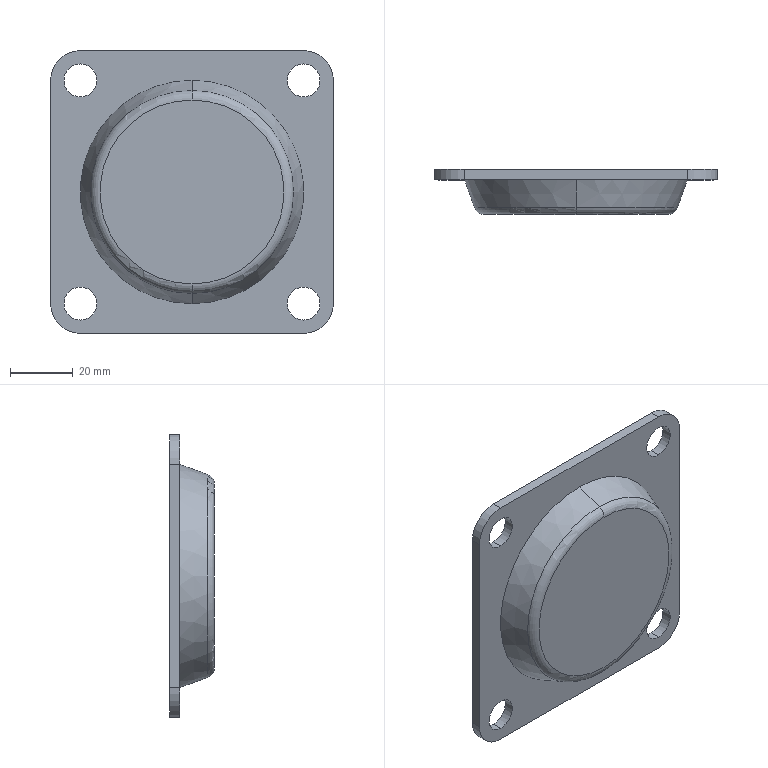Part | SolidWorks | features RefAxis 6, 3DProfileFeature 2, ICE 2, Extrusion 1, Revolution 1 | 1 solid | 29 faces | box 90 x 14.2 x 90 mm | volume 60346 mm3 | cylinder 16 | plane 9 | cone 2 | torus 2 | commonest cylinder face diameters 10.5 x8 19 x4 27 x2 54 x2
STEP:
#1=CARTESIAN_POINT('',(0.,-12.094,32.263));
#2=VERTEX_POINT('',#1);
#3=CARTESIAN_POINT('',(0.,-12.094,-32.263));
#4=VERTEX_POINT('',#3);
#5=CARTESIAN_POINT('',(0.,-12.094,0.));
#6=DIRECTION('',(0.,1.,0.));
#7=DIRECTION('',(0.,0.,1.));
#8=AXIS2_PLACEMENT_3D('',#5,#6,#7);
#9=CIRCLE('',#8,32.263);
#10=EDGE_CURVE('',#2,#4,#9,.T.);
#11=ORIENTED_EDGE('',*,*,#10,.T.);
#12=CARTESIAN_POINT('',(0.,-3.2,-35.5));
#13=VERTEX_POINT('',#12);
#14=CARTESIAN_POINT('',(0.,-3.2,-35.5));
#15=DIRECTION('',(0.,0.9397,-0.342));
#16=VECTOR('',#15,1000.);
#17=LINE('',#14,#16);
#18=EDGE_CURVE('',#4,#13,#17,.T.);
#19=ORIENTED_EDGE('',*,*,#18,.T.);
#20=CARTESIAN_POINT('',(0.,-3.2,35.5));
#21=VERTEX_POINT('',#20);
#22=CARTESIAN_POINT('',(0.,-3.2,0.));
#23=DIRECTION('',(0.,1.,0.));
#24=DIRECTION('',(0.,0.,1.));
#25=AXIS2_PLACEMENT_3D('',#22,#23,#24);
#26=CIRCLE('',#25,35.5);
#27=EDGE_CURVE('',#21,#13,#26,.T.);
#28=ORIENTED_EDGE('',*,*,#27,.F.);
#29=CARTESIAN_POINT('',(0.,-3.2,35.5));
#30=DIRECTION('',(0.,0.9397,0.342));
#31=VECTOR('',#30,1000.);
#32=LINE('',#29,#31);
#33=EDGE_CURVE('',#2,#21,#32,.T.);
#34=ORIENTED_EDGE('',*,*,#33,.F.);
#35=EDGE_LOOP('',(#11,#19,#28,#34));
#36=FACE_OUTER_BOUND('',#35,.T.);
#37=CARTESIAN_POINT('',(0.,-3.2,0.));
#38=DIRECTION('',(0.,1.,0.));
#39=DIRECTION('',(0.,0.,1.));
#40=AXIS2_PLACEMENT_3D('',#37,#38,#39);
#41=CONICAL_SURFACE('',#40,35.5,0.3491);
#42=ADVANCED_FACE('',(#36),#41,.T.);
#43=CARTESIAN_POINT('',(0.,-14.2,29.256));
#44=VERTEX_POINT('',#43);
#45=CARTESIAN_POINT('',(0.,-14.2,-29.256));
#46=VERTEX_POINT('',#45);
#47=CARTESIAN_POINT('',(0.,-14.2,0.));
#48=DIRECTION('',(0.,1.,0.));
#49=DIRECTION('',(0.,0.,1.));
#50=AXIS2_PLACEMENT_3D('',#47,#48,#49);
#51=CIRCLE('',#50,29.256);
#52=EDGE_CURVE('',#44,#46,#51,.T.);
#53=ORIENTED_EDGE('',*,*,#52,.T.);
#54=CARTESIAN_POINT('',(0.,-11.,-29.256));
#55=DIRECTION('',(1.,0.,0.));
#56=DIRECTION('',(0.,0.,-1.));
#57=AXIS2_PLACEMENT_3D('',#54,#55,#56);
#58=CIRCLE('',#57,3.2);
#59=EDGE_CURVE('',#46,#4,#58,.T.);
#60=ORIENTED_EDGE('',*,*,#59,.T.);
#61=ORIENTED_EDGE('',*,*,#10,.F.);
#62=CARTESIAN_POINT('',(0.,-11.,29.256));
#63=DIRECTION('',(-1.,0.,0.));
#64=DIRECTION('',(0.,0.,1.));
#65=AXIS2_PLACEMENT_3D('',#62,#63,#64);
#66=CIRCLE('',#65,3.2);
#67=EDGE_CURVE('',#44,#2,#66,.T.);
#68=ORIENTED_EDGE('',*,*,#67,.F.);
#69=EDGE_LOOP('',(#53,#60,#61,#68));
#70=FACE_OUTER_BOUND('',#69,.T.);
#71=CARTESIAN_POINT('',(0.,-11.,0.));
#72=DIRECTION('',(0.,1.,0.));
#73=DIRECTION('',(0.,0.,1.));
#74=AXIS2_PLACEMENT_3D('',#71,#72,#73);
#75=TOROIDAL_SURFACE('',#74,29.256,3.2);
#76=ADVANCED_FACE('',(#70),#75,.T.);
#77=CARTESIAN_POINT('',(0.,-0.5,13.5));
#78=VERTEX_POINT('',#77);
#79=CARTESIAN_POINT('',(0.,-0.5,-13.5));
#80=VERTEX_POINT('',#79);
#81=CARTESIAN_POINT('',(0.,-0.5,0.));
#82=DIRECTION('',(0.,1.,0.));
#83=DIRECTION('',(0.,0.,1.));
#84=AXIS2_PLACEMENT_3D('',#81,#82,#83);
#85=CIRCLE('',#84,13.5);
#86=EDGE_CURVE('',#78,#80,#85,.T.);
#87=ORIENTED_EDGE('',*,*,#86,.F.);
#88=CARTESIAN_POINT('',(0.,-1.5,13.5));
#89=VERTEX_POINT('',#88);
#90=CARTESIAN_POINT('',(0.,-0.5,13.5));
#91=DIRECTION('',(0.,-1.,0.));
#92=VECTOR('',#91,1000.);
#93=LINE('',#90,#92);
#94=EDGE_CURVE('',#78,#89,#93,.T.);
#95=ORIENTED_EDGE('',*,*,#94,.T.);
#96=CARTESIAN_POINT('',(0.,-1.5,-13.5));
#97=VERTEX_POINT('',#96);
#98=CARTESIAN_POINT('',(0.,-1.5,0.));
#99=DIRECTION('',(0.,1.,0.));
#100=DIRECTION('',(0.,0.,1.));
#101=AXIS2_PLACEMENT_3D('',#98,#99,#100);
#102=CIRCLE('',#101,13.5);
#103=EDGE_CURVE('',#89,#97,#102,.T.);
#104=ORIENTED_EDGE('',*,*,#103,.T.);
#105=CARTESIAN_POINT('',(0.,-0.5,-13.5));
#106=DIRECTION('',(0.,-1.,0.));
#107=VECTOR('',#106,1000.);
#108=LINE('',#105,#107);
#109=EDGE_CURVE('',#80,#97,#108,.T.);
#110=ORIENTED_EDGE('',*,*,#109,.F.);
#111=EDGE_LOOP('',(#87,#95,#104,#110));
#112=FACE_OUTER_BOUND('',#111,.T.);
#113=CARTESIAN_POINT('',(0.,-0.5,0.));
#114=DIRECTION('',(0.,-1.,0.));
#115=DIRECTION('',(0.,0.,-1.));
#116=AXIS2_PLACEMENT_3D('',#113,#114,#115);
#117=CYLINDRICAL_SURFACE('',#116,13.5);
#118=ADVANCED_FACE('',(#112),#117,.T.);
#119=CARTESIAN_POINT('',(0.,-1.5,-27.));
#120=VERTEX_POINT('',#119);
#121=CARTESIAN_POINT('',(0.,-1.5,27.));
#122=VERTEX_POINT('',#121);
#123=CARTESIAN_POINT('',(0.,-1.5,0.));
#124=DIRECTION('',(0.,1.,0.));
#125=DIRECTION('',(0.,0.,1.));
#126=AXIS2_PLACEMENT_3D('',#123,#124,#125);
#127=CIRCLE('',#126,27.);
#128=EDGE_CURVE('',#120,#122,#127,.T.);
#129=ORIENTED_EDGE('',*,*,#128,.F.);
#130=CARTESIAN_POINT('',(0.,0.,-27.));
#131=VERTEX_POINT('',#130);
#132=CARTESIAN_POINT('',(0.,-1.5,-27.));
#133=DIRECTION('',(0.,1.,0.));
#134=VECTOR('',#133,1000.);
#135=LINE('',#132,#134);
#136=EDGE_CURVE('',#120,#131,#135,.T.);
#137=ORIENTED_EDGE('',*,*,#136,.T.);
#138=CARTESIAN_POINT('',(0.,0.,27.));
#139=VERTEX_POINT('',#138);
#140=CARTESIAN_POINT('',(0.,0.,0.));
#141=DIRECTION('',(0.,1.,0.));
#142=DIRECTION('',(0.,0.,1.));
#143=AXIS2_PLACEMENT_3D('',#140,#141,#142);
#144=CIRCLE('',#143,27.);
#145=EDGE_CURVE('',#131,#139,#144,.T.);
#146=ORIENTED_EDGE('',*,*,#145,.T.);
#147=CARTESIAN_POINT('',(0.,-1.5,27.));
#148=DIRECTION('',(0.,1.,0.));
#149=VECTOR('',#148,1000.);
#150=LINE('',#147,#149);
#151=EDGE_CURVE('',#122,#139,#150,.T.);
#152=ORIENTED_EDGE('',*,*,#151,.F.);
#153=EDGE_LOOP('',(#129,#137,#146,#152));
#154=FACE_OUTER_BOUND('',#153,.T.);
#155=CARTESIAN_POINT('',(0.,-1.5,0.));
#156=DIRECTION('',(0.,1.,0.));
#157=DIRECTION('',(0.,0.,1.));
#158=AXIS2_PLACEMENT_3D('',#155,#156,#157);
#159=CYLINDRICAL_SURFACE('',#158,27.);
#160=ADVANCED_FACE('',(#154),#159,.F.);
#161=CARTESIAN_POINT('',(-35.5,-3.2,-40.75));
#162=VERTEX_POINT('',#161);
#163=CARTESIAN_POINT('',(-35.5,-3.2,-30.25));
#164=VERTEX_POINT('',#163);
#165=CARTESIAN_POINT('',(-35.5,-3.2,-35.5));
#166=DIRECTION('',(0.,1.,0.));
#167=DIRECTION('',(0.,0.,1.));
#168=AXIS2_PLACEMENT_3D('',#165,#166,#167);
#169=CIRCLE('',#168,5.25);
#170=EDGE_CURVE('',#162,#164,#169,.T.);
#171=ORIENTED_EDGE('',*,*,#170,.F.);
#172=CARTESIAN_POINT('',(-35.5,0.,-40.75));
#173=VERTEX_POINT('',#172);
#174=CARTESIAN_POINT('',(-35.5,-3.2,-40.75));
#175=DIRECTION('',(0.,1.,0.));
#176=VECTOR('',#175,1000.);
#177=LINE('',#174,#176);
#178=EDGE_CURVE('',#162,#173,#177,.T.);
#179=ORIENTED_EDGE('',*,*,#178,.T.);
#180=CARTESIAN_POINT('',(-35.5,0.,-30.25));
#181=VERTEX_POINT('',#180);
#182=CARTESIAN_POINT('',(-35.5,0.,-35.5));
#183=DIRECTION('',(0.,1.,0.));
#184=DIRECTION('',(0.,0.,1.));
#185=AXIS2_PLACEMENT_3D('',#182,#183,#184);
#186=CIRCLE('',#185,5.25);
#187=EDGE_CURVE('',#173,#181,#186,.T.);
#188=ORIENTED_EDGE('',*,*,#187,.T.);
#189=CARTESIAN_POINT('',(-35.5,-3.2,-30.25));
#190=DIRECTION('',(0.,1.,0.));
#191=VECTOR('',#190,1000.);
#192=LINE('',#189,#191);
#193=EDGE_CURVE('',#164,#181,#192,.T.);
#194=ORIENTED_EDGE('',*,*,#193,.F.);
#195=EDGE_LOOP('',(#171,#179,#188,#194));
#196=FACE_OUTER_BOUND('',#195,.T.);
#197=CARTESIAN_POINT('',(-35.5,-3.2,-35.5));
#198=DIRECTION('',(0.,1.,0.));
#199=DIRECTION('',(0.,0.,1.));
#200=AXIS2_PLACEMENT_3D('',#197,#198,#199);
#201=CYLINDRICAL_SURFACE('',#200,5.25);
#202=ADVANCED_FACE('',(#196),#201,.F.);
#203=CARTESIAN_POINT('',(-35.5,-3.2,30.25));
#204=VERTEX_POINT('',#203);
#205=CARTESIAN_POINT('',(-35.5,-3.2,40.75));
#206=VERTEX_POINT('',#205);
#207=CARTESIAN_POINT('',(-35.5,-3.2,35.5));
#208=DIRECTION('',(0.,1.,0.));
#209=DIRECTION('',(0.,0.,1.));
#210=AXIS2_PLACEMENT_3D('',#207,#208,#209);
#211=CIRCLE('',#210,5.25);
#212=EDGE_CURVE('',#204,#206,#211,.T.);
#213=ORIENTED_EDGE('',*,*,#212,.F.);
#214=CARTESIAN_POINT('',(-35.5,0.,30.25));
#215=VERTEX_POINT('',#214);
#216=CARTESIAN_POINT('',(-35.5,-3.2,30.25));
#217=DIRECTION('',(0.,1.,0.));
#218=VECTOR('',#217,1000.);
#219=LINE('',#216,#218);
#220=EDGE_CURVE('',#204,#215,#219,.T.);
#221=ORIENTED_EDGE('',*,*,#220,.T.);
#222=CARTESIAN_POINT('',(-35.5,0.,40.75));
#223=VERTEX_POINT('',#222);
#224=CARTESIAN_POINT('',(-35.5,0.,35.5));
#225=DIRECTION('',(0.,1.,0.));
#226=DIRECTION('',(0.,0.,1.));
#227=AXIS2_PLACEMENT_3D('',#224,#225,#226);
#228=CIRCLE('',#227,5.25);
#229=EDGE_CURVE('',#215,#223,#228,.T.);
#230=ORIENTED_EDGE('',*,*,#229,.T.);
#231=CARTESIAN_POINT('',(-35.5,-3.2,40.75));
#232=DIRECTION('',(0.,1.,0.));
#233=VECTOR('',#232,1000.);
#234=LINE('',#231,#233);
#235=EDGE_CURVE('',#206,#223,#234,.T.);
#236=ORIENTED_EDGE('',*,*,#235,.F.);
#237=EDGE_LOOP('',(#213,#221,#230,#236));
#238=FACE_OUTER_BOUND('',#237,.T.);
#239=CARTESIAN_POINT('',(-35.5,-3.2,35.5));
#240=DIRECTION('',(0.,1.,0.));
#241=DIRECTION('',(0.,0.,1.));
#242=AXIS2_PLACEMENT_3D('',#239,#240,#241);
#243=CYLINDRICAL_SURFACE('',#242,5.25);
#244=ADVANCED_FACE('',(#238),#243,.F.);
#245=CARTESIAN_POINT('',(35.5,-3.2,-40.75));
#246=VERTEX_POINT('',#245);
#247=CARTESIAN_POINT('',(35.5,-3.2,-30.25));
#248=VERTEX_POINT('',#247);
#249=CARTESIAN_POINT('',(35.5,-3.2,-35.5));
#250=DIRECTION('',(0.,1.,0.));
#251=DIRECTION('',(0.,0.,1.));
#252=AXIS2_PLACEMENT_3D('',#249,#250,#251);
#253=CIRCLE('',#252,5.25);
#254=EDGE_CURVE('',#246,#248,#253,.T.);
#255=ORIENTED_EDGE('',*,*,#254,.F.);
#256=CARTESIAN_POINT('',(35.5,0.,-40.75));
#257=VERTEX_POINT('',#256);
#258=CARTESIAN_POINT('',(35.5,-3.2,-40.75));
#259=DIRECTION('',(0.,1.,0.));
#260=VECTOR('',#259,1000.);
#261=LINE('',#258,#260);
#262=EDGE_CURVE('',#246,#257,#261,.T.);
#263=ORIENTED_EDGE('',*,*,#262,.T.);
#264=CARTESIAN_POINT('',(35.5,0.,-30.25));
#265=VERTEX_POINT('',#264);
#266=CARTESIAN_POINT('',(35.5,0.,-35.5));
#267=DIRECTION('',(0.,1.,0.));
#268=DIRECTION('',(0.,0.,1.));
#269=AXIS2_PLACEMENT_3D('',#266,#267,#268);
#270=CIRCLE('',#269,5.25);
#271=EDGE_CURVE('',#257,#265,#270,.T.);
#272=ORIENTED_EDGE('',*,*,#271,.T.);
#273=CARTESIAN_POINT('',(35.5,-3.2,-30.25));
#274=DIRECTION('',(0.,1.,0.));
#275=VECTOR('',#274,1000.);
#276=LINE('',#273,#275);
#277=EDGE_CURVE('',#248,#265,#276,.T.);
#278=ORIENTED_EDGE('',*,*,#277,.F.);
#279=EDGE_LOOP('',(#255,#263,#272,#278));
#280=FACE_OUTER_BOUND('',#279,.T.);
#281=CARTESIAN_POINT('',(35.5,-3.2,-35.5));
#282=DIRECTION('',(0.,1.,0.));
#283=DIRECTION('',(0.,0.,1.));
#284=AXIS2_PLACEMENT_3D('',#281,#282,#283);
#285=CYLINDRICAL_SURFACE('',#284,5.25);
#286=ADVANCED_FACE('',(#280),#285,.F.);
#287=CARTESIAN_POINT('',(35.5,-3.2,30.25));
#288=VERTEX_POINT('',#287);
#289=CARTESIAN_POINT('',(35.5,-3.2,40.75));
#290=VERTEX_POINT('',#289);
#291=CARTESIAN_POINT('',(35.5,-3.2,35.5));
#292=DIRECTION('',(0.,1.,0.));
#293=DIRECTION('',(0.,0.,1.));
#294=AXIS2_PLACEMENT_3D('',#291,#292,#293);
#295=CIRCLE('',#294,5.25);
#296=EDGE_CURVE('',#288,#290,#295,.T.);
#297=ORIENTED_EDGE('',*,*,#296,.F.);
#298=CARTESIAN_POINT('',(35.5,0.,30.25));
#299=VERTEX_POINT('',#298);
#300=CARTESIAN_POINT('',(35.5,-3.2,30.25));
#301=DIRECTION('',(0.,1.,0.));
#302=VECTOR('',#301,1000.);
#303=LINE('',#300,#302);
#304=EDGE_CURVE('',#288,#299,#303,.T.);
#305=ORIENTED_EDGE('',*,*,#304,.T.);
#306=CARTESIAN_POINT('',(35.5,0.,40.75));
#307=VERTEX_POINT('',#306);
#308=CARTESIAN_POINT('',(35.5,0.,35.5));
#309=DIRECTION('',(0.,1.,0.));
#310=DIRECTION('',(0.,0.,1.));
#311=AXIS2_PLACEMENT_3D('',#308,#309,#310);
#312=CIRCLE('',#311,5.25);
#313=EDGE_CURVE('',#299,#307,#312,.T.);
#314=ORIENTED_EDGE('',*,*,#313,.T.);
#315=CARTESIAN_POINT('',(35.5,-3.2,40.75));
#316=DIRECTION('',(0.,1.,0.));
#317=VECTOR('',#316,1000.);
#318=LINE('',#315,#317);
#319=EDGE_CURVE('',#290,#307,#318,.T.);
#320=ORIENTED_EDGE('',*,*,#319,.F.);
#321=EDGE_LOOP('',(#297,#305,#314,#320));
#322=FACE_OUTER_BOUND('',#321,.T.);
#323=CARTESIAN_POINT('',(35.5,-3.2,35.5));
#324=DIRECTION('',(0.,1.,0.));
#325=DIRECTION('',(0.,0.,1.));
#326=AXIS2_PLACEMENT_3D('',#323,#324,#325);
#327=CYLINDRICAL_SURFACE('',#326,5.25);
#328=ADVANCED_FACE('',(#322),#327,.F.);
#329=CARTESIAN_POINT('',(-45.,0.,35.5));
#330=VERTEX_POINT('',#329);
#331=CARTESIAN_POINT('',(-35.5,0.,45.));
#332=VERTEX_POINT('',#331);
#333=CARTESIAN_POINT('',(-35.5,0.,35.5));
#334=DIRECTION('',(0.,1.,0.));
#335=DIRECTION('',(0.,0.,1.));
#336=AXIS2_PLACEMENT_3D('',#333,#334,#335);
#337=CIRCLE('',#336,9.5);
#338=EDGE_CURVE('',#330,#332,#337,.T.);
#339=ORIENTED_EDGE('',*,*,#338,.F.);
#340=CARTESIAN_POINT('',(-45.,-3.2,35.5));
#341=VERTEX_POINT('',#340);
#342=CARTESIAN_POINT('',(-45.,-3.2,35.5));
#343=DIRECTION('',(0.,1.,0.));
#344=VECTOR('',#343,1000.);
#345=LINE('',#342,#344);
#346=EDGE_CURVE('',#341,#330,#345,.T.);
#347=ORIENTED_EDGE('',*,*,#346,.F.);
#348=CARTESIAN_POINT('',(-35.5,-3.2,45.));
#349=VERTEX_POINT('',#348);
#350=CARTESIAN_POINT('',(-35.5,-3.2,35.5));
#351=DIRECTION('',(0.,1.,0.));
#352=DIRECTION('',(0.,0.,1.));
#353=AXIS2_PLACEMENT_3D('',#350,#351,#352);
#354=CIRCLE('',#353,9.5);
#355=EDGE_CURVE('',#341,#349,#354,.T.);
#356=ORIENTED_EDGE('',*,*,#355,.T.);
#357=CARTESIAN_POINT('',(-35.5,-3.2,45.));
#358=DIRECTION('',(0.,1.,0.));
#359=VECTOR('',#358,1000.);
#360=LINE('',#357,#359);
#361=EDGE_CURVE('',#349,#332,#360,.T.);
#362=ORIENTED_EDGE('',*,*,#361,.T.);
#363=EDGE_LOOP('',(#339,#347,#356,#362));
#364=FACE_OUTER_BOUND('',#363,.T.);
#365=CARTESIAN_POINT('',(-35.5,-3.2,35.5));
#366=DIRECTION('',(0.,1.,0.));
#367=DIRECTION('',(0.,0.,1.));
#368=AXIS2_PLACEMENT_3D('',#365,#366,#367);
#369=CYLINDRICAL_SURFACE('',#368,9.5);
#370=ADVANCED_FACE('',(#364),#369,.T.);
#371=CARTESIAN_POINT('',(-45.,0.,-35.5));
#372=VERTEX_POINT('',#371);
#373=CARTESIAN_POINT('',(-45.,0.,-35.5));
#374=DIRECTION('',(0.,0.,1.));
#375=VECTOR('',#374,1000.);
#376=LINE('',#373,#375);
#377=EDGE_CURVE('',#372,#330,#376,.T.);
#378=ORIENTED_EDGE('',*,*,#377,.F.);
#379=CARTESIAN_POINT('',(-45.,-3.2,-35.5));
#380=VERTEX_POINT('',#379);
#381=CARTESIAN_POINT('',(-45.,-3.2,-35.5));
#382=DIRECTION('',(0.,1.,0.));
#383=VECTOR('',#382,1000.);
#384=LINE('',#381,#383);
#385=EDGE_CURVE('',#380,#372,#384,.T.);
#386=ORIENTED_EDGE('',*,*,#385,.F.);
#387=CARTESIAN_POINT('',(-45.,-3.2,-35.5));
#388=DIRECTION('',(0.,0.,1.));
#389=VECTOR('',#388,1000.);
#390=LINE('',#387,#389);
#391=EDGE_CURVE('',#380,#341,#390,.T.);
#392=ORIENTED_EDGE('',*,*,#391,.T.);
#393=ORIENTED_EDGE('',*,*,#346,.T.);
#394=EDGE_LOOP('',(#378,#386,#392,#393));
#395=FACE_OUTER_BOUND('',#394,.T.);
#396=CARTESIAN_POINT('',(-45.,-3.2,-35.5));
#397=DIRECTION('',(-1.,0.,0.));
#398=DIRECTION('',(0.,0.,1.));
#399=AXIS2_PLACEMENT_3D('',#396,#397,#398);
#400=PLANE('',#399);
#401=ADVANCED_FACE('',(#395),#400,.T.);
#402=CARTESIAN_POINT('',(-35.5,0.,-45.));
#403=VERTEX_POINT('',#402);
#404=CARTESIAN_POINT('',(-35.5,0.,-35.5));
#405=DIRECTION('',(0.,1.,0.));
#406=DIRECTION('',(0.,0.,1.));
#407=AXIS2_PLACEMENT_3D('',#404,#405,#406);
#408=CIRCLE('',#407,9.5);
#409=EDGE_CURVE('',#403,#372,#408,.T.);
#410=ORIENTED_EDGE('',*,*,#409,.F.);
#411=CARTESIAN_POINT('',(-35.5,-3.2,-45.));
#412=VERTEX_POINT('',#411);
#413=CARTESIAN_POINT('',(-35.5,-3.2,-45.));
#414=DIRECTION('',(0.,1.,0.));
#415=VECTOR('',#414,1000.);
#416=LINE('',#413,#415);
#417=EDGE_CURVE('',#412,#403,#416,.T.);
#418=ORIENTED_EDGE('',*,*,#417,.F.);
#419=CARTESIAN_POINT('',(-35.5,-3.2,-35.5));
#420=DIRECTION('',(0.,1.,0.));
#421=DIRECTION('',(0.,0.,1.));
#422=AXIS2_PLACEMENT_3D('',#419,#420,#421);
#423=CIRCLE('',#422,9.5);
#424=EDGE_CURVE('',#412,#380,#423,.T.);
#425=ORIENTED_EDGE('',*,*,#424,.T.);
#426=ORIENTED_EDGE('',*,*,#385,.T.);
#427=EDGE_LOOP('',(#410,#418,#425,#426));
#428=FACE_OUTER_BOUND('',#427,.T.);
#429=CARTESIAN_POINT('',(-35.5,-3.2,-35.5));
#430=DIRECTION('',(0.,1.,0.));
#431=DIRECTION('',(0.,0.,1.));
#432=AXIS2_PLACEMENT_3D('',#429,#430,#431);
#433=CYLINDRICAL_SURFACE('',#432,9.5);
#434=ADVANCED_FACE('',(#428),#433,.T.);
#435=CARTESIAN_POINT('',(35.5,0.,-45.));
#436=VERTEX_POINT('',#435);
#437=CARTESIAN_POINT('',(35.5,0.,-45.));
#438=DIRECTION('',(-1.,0.,0.));
#439=VECTOR('',#438,1000.);
#440=LINE('',#437,#439);
#441=EDGE_CURVE('',#436,#403,#440,.T.);
#442=ORIENTED_EDGE('',*,*,#441,.F.);
#443=CARTESIAN_POINT('',(35.5,-3.2,-45.));
#444=VERTEX_POINT('',#443);
#445=CARTESIAN_POINT('',(35.5,-3.2,-45.));
#446=DIRECTION('',(0.,1.,0.));
#447=VECTOR('',#446,1000.);
#448=LINE('',#445,#447);
#449=EDGE_CURVE('',#444,#436,#448,.T.);
#450=ORIENTED_EDGE('',*,*,#449,.F.);
#451=CARTESIAN_POINT('',(35.5,-3.2,-45.));
#452=DIRECTION('',(-1.,0.,0.));
#453=VECTOR('',#452,1000.);
#454=LINE('',#451,#453);
#455=EDGE_CURVE('',#444,#412,#454,.T.);
#456=ORIENTED_EDGE('',*,*,#455,.T.);
#457=ORIENTED_EDGE('',*,*,#417,.T.);
#458=EDGE_LOOP('',(#442,#450,#456,#457));
#459=FACE_OUTER_BOUND('',#458,.T.);
#460=CARTESIAN_POINT('',(35.5,-3.2,-45.));
#461=DIRECTION('',(0.,0.,-1.));
#462=DIRECTION('',(-1.,0.,0.));
#463=AXIS2_PLACEMENT_3D('',#460,#461,#462);
#464=PLANE('',#463);
#465=ADVANCED_FACE('',(#459),#464,.T.);
#466=CARTESIAN_POINT('',(45.,0.,-35.5));
#467=VERTEX_POINT('',#466);
#468=CARTESIAN_POINT('',(35.5,0.,-35.5));
#469=DIRECTION('',(0.,1.,0.));
#470=DIRECTION('',(0.,0.,1.));
#471=AXIS2_PLACEMENT_3D('',#468,#469,#470);
#472=CIRCLE('',#471,9.5);
#473=EDGE_CURVE('',#467,#436,#472,.T.);
#474=ORIENTED_EDGE('',*,*,#473,.F.);
#475=CARTESIAN_POINT('',(45.,-3.2,-35.5));
#476=VERTEX_POINT('',#475);
#477=CARTESIAN_POINT('',(45.,-3.2,-35.5));
#478=DIRECTION('',(0.,1.,0.));
#479=VECTOR('',#478,1000.);
#480=LINE('',#477,#479);
#481=EDGE_CURVE('',#476,#467,#480,.T.);
#482=ORIENTED_EDGE('',*,*,#481,.F.);
#483=CARTESIAN_POINT('',(35.5,-3.2,-35.5));
#484=DIRECTION('',(0.,1.,0.));
#485=DIRECTION('',(0.,0.,1.));
#486=AXIS2_PLACEMENT_3D('',#483,#484,#485);
#487=CIRCLE('',#486,9.5);
#488=EDGE_CURVE('',#476,#444,#487,.T.);
#489=ORIENTED_EDGE('',*,*,#488,.T.);
#490=ORIENTED_EDGE('',*,*,#449,.T.);
#491=EDGE_LOOP('',(#474,#482,#489,#490));
#492=FACE_OUTER_BOUND('',#491,.T.);
#493=CARTESIAN_POINT('',(35.5,-3.2,-35.5));
#494=DIRECTION('',(0.,1.,0.));
#495=DIRECTION('',(0.,0.,1.));
#496=AXIS2_PLACEMENT_3D('',#493,#494,#495);
#497=CYLINDRICAL_SURFACE('',#496,9.5);
#498=ADVANCED_FACE('',(#492),#497,.T.);
#499=CARTESIAN_POINT('',(45.,0.,35.5));
#500=VERTEX_POINT('',#499);
#501=CARTESIAN_POINT('',(45.,0.,35.5));
#502=DIRECTION('',(0.,0.,-1.));
#503=VECTOR('',#502,1000.);
#504=LINE('',#501,#503);
#505=EDGE_CURVE('',#500,#467,#504,.T.);
#506=ORIENTED_EDGE('',*,*,#505,.F.);
#507=CARTESIAN_POINT('',(45.,-3.2,35.5));
#508=VERTEX_POINT('',#507);
#509=CARTESIAN_POINT('',(45.,-3.2,35.5));
#510=DIRECTION('',(0.,1.,0.));
#511=VECTOR('',#510,1000.);
#512=LINE('',#509,#511);
#513=EDGE_CURVE('',#508,#500,#512,.T.);
#514=ORIENTED_EDGE('',*,*,#513,.F.);
#515=CARTESIAN_POINT('',(45.,-3.2,35.5));
#516=DIRECTION('',(0.,0.,-1.));
#517=VECTOR('',#516,1000.);
#518=LINE('',#515,#517);
#519=EDGE_CURVE('',#508,#476,#518,.T.);
#520=ORIENTED_EDGE('',*,*,#519,.T.);
#521=ORIENTED_EDGE('',*,*,#481,.T.);
#522=EDGE_LOOP('',(#506,#514,#520,#521));
#523=FACE_OUTER_BOUND('',#522,.T.);
#524=CARTESIAN_POINT('',(45.,-3.2,35.5));
#525=DIRECTION('',(1.,0.,0.));
#526=DIRECTION('',(0.,0.,-1.));
#527=AXIS2_PLACEMENT_3D('',#524,#525,#526);
#528=PLANE('',#527);
#529=ADVANCED_FACE('',(#523),#528,.T.);
#530=CARTESIAN_POINT('',(35.5,0.,45.));
#531=VERTEX_POINT('',#530);
#532=CARTESIAN_POINT('',(35.5,0.,35.5));
#533=DIRECTION('',(0.,1.,0.));
#534=DIRECTION('',(0.,0.,1.));
#535=AXIS2_PLACEMENT_3D('',#532,#533,#534);
#536=CIRCLE('',#535,9.5);
#537=EDGE_CURVE('',#531,#500,#536,.T.);
#538=ORIENTED_EDGE('',*,*,#537,.F.);
#539=CARTESIAN_POINT('',(35.5,-3.2,45.));
#540=VERTEX_POINT('',#539);
#541=CARTESIAN_POINT('',(35.5,-3.2,45.));
#542=DIRECTION('',(0.,1.,0.));
#543=VECTOR('',#542,1000.);
#544=LINE('',#541,#543);
#545=EDGE_CURVE('',#540,#531,#544,.T.);
#546=ORIENTED_EDGE('',*,*,#545,.F.);
#547=CARTESIAN_POINT('',(35.5,-3.2,35.5));
#548=DIRECTION('',(0.,1.,0.));
#549=DIRECTION('',(0.,0.,1.));
#550=AXIS2_PLACEMENT_3D('',#547,#548,#549);
#551=CIRCLE('',#550,9.5);
#552=EDGE_CURVE('',#540,#508,#551,.T.);
#553=ORIENTED_EDGE('',*,*,#552,.T.);
#554=ORIENTED_EDGE('',*,*,#513,.T.);
#555=EDGE_LOOP('',(#538,#546,#553,#554));
#556=FACE_OUTER_BOUND('',#555,.T.);
#557=CARTESIAN_POINT('',(35.5,-3.2,35.5));
#558=DIRECTION('',(0.,1.,0.));
#559=DIRECTION('',(0.,0.,1.));
#560=AXIS2_PLACEMENT_3D('',#557,#558,#559);
#561=CYLINDRICAL_SURFACE('',#560,9.5);
#562=ADVANCED_FACE('',(#556),#561,.T.);
#563=CARTESIAN_POINT('',(-35.5,0.,45.));
#564=DIRECTION('',(1.,0.,0.));
#565=VECTOR('',#564,1000.);
#566=LINE('',#563,#565);
#567=EDGE_CURVE('',#332,#531,#566,.T.);
#568=ORIENTED_EDGE('',*,*,#567,.F.);
#569=ORIENTED_EDGE('',*,*,#361,.F.);
#570=CARTESIAN_POINT('',(-35.5,-3.2,45.));
#571=DIRECTION('',(1.,0.,0.));
#572=VECTOR('',#571,1000.);
#573=LINE('',#570,#572);
#574=EDGE_CURVE('',#349,#540,#573,.T.);
#575=ORIENTED_EDGE('',*,*,#574,.T.);
#576=ORIENTED_EDGE('',*,*,#545,.T.);
#577=EDGE_LOOP('',(#568,#569,#575,#576));
#578=FACE_OUTER_BOUND('',#577,.T.);
#579=CARTESIAN_POINT('',(-35.5,-3.2,45.));
#580=DIRECTION('',(0.,0.,1.));
#581=DIRECTION('',(1.,0.,0.));
#582=AXIS2_PLACEMENT_3D('',#579,#580,#581);
#583=PLANE('',#582);
#584=ADVANCED_FACE('',(#578),#583,.T.);
#585=ORIENTED_EDGE('',*,*,#27,.T.);
#586=CARTESIAN_POINT('',(0.,-3.2,0.));
#587=DIRECTION('',(0.,1.,0.));
#588=DIRECTION('',(0.,0.,1.));
#589=AXIS2_PLACEMENT_3D('',#586,#587,#588);
#590=CIRCLE('',#589,35.5);
#591=EDGE_CURVE('',#13,#21,#590,.T.);
#592=ORIENTED_EDGE('',*,*,#591,.T.);
#593=EDGE_LOOP('',(#585,#592));
#594=FACE_BOUND('',#593,.T.);
#595=CARTESIAN_POINT('',(-35.5,-3.2,-35.5));
#596=DIRECTION('',(0.,1.,0.));
#597=DIRECTION('',(0.,0.,1.));
#598=AXIS2_PLACEMENT_3D('',#595,#596,#597);
#599=CIRCLE('',#598,5.25);
#600=EDGE_CURVE('',#164,#162,#599,.T.);
#601=ORIENTED_EDGE('',*,*,#600,.T.);
#602=ORIENTED_EDGE('',*,*,#170,.T.);
#603=EDGE_LOOP('',(#601,#602));
#604=FACE_BOUND('',#603,.T.);
#605=CARTESIAN_POINT('',(-35.5,-3.2,35.5));
#606=DIRECTION('',(0.,1.,0.));
#607=DIRECTION('',(0.,0.,1.));
#608=AXIS2_PLACEMENT_3D('',#605,#606,#607);
#609=CIRCLE('',#608,5.25);
#610=EDGE_CURVE('',#206,#204,#609,.T.);
#611=ORIENTED_EDGE('',*,*,#610,.T.);
#612=ORIENTED_EDGE('',*,*,#212,.T.);
#613=EDGE_LOOP('',(#611,#612));
#614=FACE_BOUND('',#613,.T.);
#615=CARTESIAN_POINT('',(35.5,-3.2,-35.5));
#616=DIRECTION('',(0.,1.,0.));
#617=DIRECTION('',(0.,0.,1.));
#618=AXIS2_PLACEMENT_3D('',#615,#616,#617);
#619=CIRCLE('',#618,5.25);
#620=EDGE_CURVE('',#248,#246,#619,.T.);
#621=ORIENTED_EDGE('',*,*,#620,.T.);
#622=ORIENTED_EDGE('',*,*,#254,.T.);
#623=EDGE_LOOP('',(#621,#622));
#624=FACE_BOUND('',#623,.T.);
#625=CARTESIAN_POINT('',(35.5,-3.2,35.5));
#626=DIRECTION('',(0.,1.,0.));
#627=DIRECTION('',(0.,0.,1.));
#628=AXIS2_PLACEMENT_3D('',#625,#626,#627);
#629=CIRCLE('',#628,5.25);
#630=EDGE_CURVE('',#290,#288,#629,.T.);
#631=ORIENTED_EDGE('',*,*,#630,.T.);
#632=ORIENTED_EDGE('',*,*,#296,.T.);
#633=EDGE_LOOP('',(#631,#632));
#634=FACE_BOUND('',#633,.T.);
#635=ORIENTED_EDGE('',*,*,#355,.F.);
#636=ORIENTED_EDGE('',*,*,#391,.F.);
#637=ORIENTED_EDGE('',*,*,#424,.F.);
#638=ORIENTED_EDGE('',*,*,#455,.F.);
#639=ORIENTED_EDGE('',*,*,#488,.F.);
#640=ORIENTED_EDGE('',*,*,#519,.F.);
#641=ORIENTED_EDGE('',*,*,#552,.F.);
#642=ORIENTED_EDGE('',*,*,#574,.F.);
#643=EDGE_LOOP('',(#635,#636,#637,#638,#639,#640,#641,#642));
#644=FACE_OUTER_BOUND('',#643,.T.);
#645=CARTESIAN_POINT('',(-35.5,-3.2,35.5));
#646=DIRECTION('',(0.,1.,0.));
#647=DIRECTION('',(0.,0.,1.));
#648=AXIS2_PLACEMENT_3D('',#645,#646,#647);
#649=PLANE('',#648);
#650=ADVANCED_FACE('',(#594,#604,#614,#624,#634,#644),#649,.F.);
#651=CARTESIAN_POINT('',(0.,0.,0.));
#652=DIRECTION('',(0.,1.,0.));
#653=DIRECTION('',(0.,0.,1.));
#654=AXIS2_PLACEMENT_3D('',#651,#652,#653);
#655=CIRCLE('',#654,27.);
#656=EDGE_CURVE('',#139,#131,#655,.T.);
#657=ORIENTED_EDGE('',*,*,#656,.F.);
#658=ORIENTED_EDGE('',*,*,#145,.F.);
#659=EDGE_LOOP('',(#657,#658));
#660=FACE_BOUND('',#659,.T.);
#661=CARTESIAN_POINT('',(-35.5,0.,-35.5));
#662=DIRECTION('',(0.,1.,0.));
#663=DIRECTION('',(0.,0.,1.));
#664=AXIS2_PLACEMENT_3D('',#661,#662,#663);
#665=CIRCLE('',#664,5.25);
#666=EDGE_CURVE('',#181,#173,#665,.T.);
#667=ORIENTED_EDGE('',*,*,#666,.F.);
#668=ORIENTED_EDGE('',*,*,#187,.F.);
#669=EDGE_LOOP('',(#667,#668));
#670=FACE_BOUND('',#669,.T.);
#671=CARTESIAN_POINT('',(-35.5,0.,35.5));
#672=DIRECTION('',(0.,1.,0.));
#673=DIRECTION('',(0.,0.,1.));
#674=AXIS2_PLACEMENT_3D('',#671,#672,#673);
#675=CIRCLE('',#674,5.25);
#676=EDGE_CURVE('',#223,#215,#675,.T.);
#677=ORIENTED_EDGE('',*,*,#676,.F.);
#678=ORIENTED_EDGE('',*,*,#229,.F.);
#679=EDGE_LOOP('',(#677,#678));
#680=FACE_BOUND('',#679,.T.);
#681=CARTESIAN_POINT('',(35.5,0.,-35.5));
#682=DIRECTION('',(0.,1.,0.));
#683=DIRECTION('',(0.,0.,1.));
#684=AXIS2_PLACEMENT_3D('',#681,#682,#683);
#685=CIRCLE('',#684,5.25);
#686=EDGE_CURVE('',#265,#257,#685,.T.);
#687=ORIENTED_EDGE('',*,*,#686,.F.);
#688=ORIENTED_EDGE('',*,*,#271,.F.);
#689=EDGE_LOOP('',(#687,#688));
#690=FACE_BOUND('',#689,.T.);
#691=CARTESIAN_POINT('',(35.5,0.,35.5));
#692=DIRECTION('',(0.,1.,0.));
#693=DIRECTION('',(0.,0.,1.));
#694=AXIS2_PLACEMENT_3D('',#691,#692,#693);
#695=CIRCLE('',#694,5.25);
#696=EDGE_CURVE('',#307,#299,#695,.T.);
#697=ORIENTED_EDGE('',*,*,#696,.F.);
#698=ORIENTED_EDGE('',*,*,#313,.F.);
#699=EDGE_LOOP('',(#697,#698));
#700=FACE_BOUND('',#699,.T.);
#701=ORIENTED_EDGE('',*,*,#338,.T.);
#702=ORIENTED_EDGE('',*,*,#567,.T.);
#703=ORIENTED_EDGE('',*,*,#537,.T.);
#704=ORIENTED_EDGE('',*,*,#505,.T.);
#705=ORIENTED_EDGE('',*,*,#473,.T.);
#706=ORIENTED_EDGE('',*,*,#441,.T.);
#707=ORIENTED_EDGE('',*,*,#409,.T.);
#708=ORIENTED_EDGE('',*,*,#377,.T.);
#709=EDGE_LOOP('',(#701,#702,#703,#704,#705,#706,#707,#708));
#710=FACE_OUTER_BOUND('',#709,.T.);
#711=CARTESIAN_POINT('',(-35.5,0.,35.5));
#712=DIRECTION('',(0.,1.,0.));
#713=DIRECTION('',(0.,0.,1.));
#714=AXIS2_PLACEMENT_3D('',#711,#712,#713);
#715=PLANE('',#714);
#716=ADVANCED_FACE('',(#660,#670,#680,#690,#700,#710),#715,.T.);
#717=ORIENTED_EDGE('',*,*,#304,.F.);
#718=ORIENTED_EDGE('',*,*,#630,.F.);
#719=ORIENTED_EDGE('',*,*,#319,.T.);
#720=ORIENTED_EDGE('',*,*,#696,.T.);
#721=EDGE_LOOP('',(#717,#718,#719,#720));
#722=FACE_OUTER_BOUND('',#721,.T.);
#723=CARTESIAN_POINT('',(35.5,-3.2,35.5));
#724=DIRECTION('',(0.,1.,0.));
#725=DIRECTION('',(0.,0.,1.));
#726=AXIS2_PLACEMENT_3D('',#723,#724,#725);
#727=CYLINDRICAL_SURFACE('',#726,5.25);
#728=ADVANCED_FACE('',(#722),#727,.F.);
#729=ORIENTED_EDGE('',*,*,#262,.F.);
#730=ORIENTED_EDGE('',*,*,#620,.F.);
#731=ORIENTED_EDGE('',*,*,#277,.T.);
#732=ORIENTED_EDGE('',*,*,#686,.T.);
#733=EDGE_LOOP('',(#729,#730,#731,#732));
#734=FACE_OUTER_BOUND('',#733,.T.);
#735=CARTESIAN_POINT('',(35.5,-3.2,-35.5));
#736=DIRECTION('',(0.,1.,0.));
#737=DIRECTION('',(0.,0.,1.));
#738=AXIS2_PLACEMENT_3D('',#735,#736,#737);
#739=CYLINDRICAL_SURFACE('',#738,5.25);
#740=ADVANCED_FACE('',(#734),#739,.F.);
#741=ORIENTED_EDGE('',*,*,#220,.F.);
#742=ORIENTED_EDGE('',*,*,#610,.F.);
#743=ORIENTED_EDGE('',*,*,#235,.T.);
#744=ORIENTED_EDGE('',*,*,#676,.T.);
#745=EDGE_LOOP('',(#741,#742,#743,#744));
#746=FACE_OUTER_BOUND('',#745,.T.);
#747=CARTESIAN_POINT('',(-35.5,-3.2,35.5));
#748=DIRECTION('',(0.,1.,0.));
#749=DIRECTION('',(0.,0.,1.));
#750=AXIS2_PLACEMENT_3D('',#747,#748,#749);
#751=CYLINDRICAL_SURFACE('',#750,5.25);
#752=ADVANCED_FACE('',(#746),#751,.F.);
#753=ORIENTED_EDGE('',*,*,#178,.F.);
#754=ORIENTED_EDGE('',*,*,#600,.F.);
#755=ORIENTED_EDGE('',*,*,#193,.T.);
#756=ORIENTED_EDGE('',*,*,#666,.T.);
#757=EDGE_LOOP('',(#753,#754,#755,#756));
#758=FACE_OUTER_BOUND('',#757,.T.);
#759=CARTESIAN_POINT('',(-35.5,-3.2,-35.5));
#760=DIRECTION('',(0.,1.,0.));
#761=DIRECTION('',(0.,0.,1.));
#762=AXIS2_PLACEMENT_3D('',#759,#760,#761);
#763=CYLINDRICAL_SURFACE('',#762,5.25);
#764=ADVANCED_FACE('',(#758),#763,.F.);
#765=ORIENTED_EDGE('',*,*,#136,.F.);
#766=CARTESIAN_POINT('',(0.,-1.5,0.));
#767=DIRECTION('',(0.,1.,0.));
#768=DIRECTION('',(0.,0.,1.));
#769=AXIS2_PLACEMENT_3D('',#766,#767,#768);
#770=CIRCLE('',#769,27.);
#771=EDGE_CURVE('',#122,#120,#770,.T.);
#772=ORIENTED_EDGE('',*,*,#771,.F.);
#773=ORIENTED_EDGE('',*,*,#151,.T.);
#774=ORIENTED_EDGE('',*,*,#656,.T.);
#775=EDGE_LOOP('',(#765,#772,#773,#774));
#776=FACE_OUTER_BOUND('',#775,.T.);
#777=CARTESIAN_POINT('',(0.,-1.5,0.));
#778=DIRECTION('',(0.,1.,0.));
#779=DIRECTION('',(0.,0.,1.));
#780=AXIS2_PLACEMENT_3D('',#777,#778,#779);
#781=CYLINDRICAL_SURFACE('',#780,27.);
#782=ADVANCED_FACE('',(#776),#781,.F.);
#783=CARTESIAN_POINT('',(0.,-1.5,0.));
#784=DIRECTION('',(0.,1.,0.));
#785=DIRECTION('',(0.,0.,1.));
#786=AXIS2_PLACEMENT_3D('',#783,#784,#785);
#787=CIRCLE('',#786,13.5);
#788=EDGE_CURVE('',#97,#89,#787,.T.);
#789=ORIENTED_EDGE('',*,*,#788,.F.);
#790=ORIENTED_EDGE('',*,*,#103,.F.);
#791=EDGE_LOOP('',(#789,#790));
#792=FACE_BOUND('',#791,.T.);
#793=ORIENTED_EDGE('',*,*,#771,.T.);
#794=ORIENTED_EDGE('',*,*,#128,.T.);
#795=EDGE_LOOP('',(#793,#794));
#796=FACE_OUTER_BOUND('',#795,.T.);
#797=CARTESIAN_POINT('',(0.,-1.5,0.));
#798=DIRECTION('',(0.,1.,0.));
#799=DIRECTION('',(0.,0.,1.));
#800=AXIS2_PLACEMENT_3D('',#797,#798,#799);
#801=PLANE('',#800);
#802=ADVANCED_FACE('',(#792,#796),#801,.T.);
#803=ORIENTED_EDGE('',*,*,#94,.F.);
#804=CARTESIAN_POINT('',(0.,-0.5,0.));
#805=DIRECTION('',(0.,1.,0.));
#806=DIRECTION('',(0.,0.,1.));
#807=AXIS2_PLACEMENT_3D('',#804,#805,#806);
#808=CIRCLE('',#807,13.5);
#809=EDGE_CURVE('',#80,#78,#808,.T.);
#810=ORIENTED_EDGE('',*,*,#809,.F.);
#811=ORIENTED_EDGE('',*,*,#109,.T.);
#812=ORIENTED_EDGE('',*,*,#788,.T.);
#813=EDGE_LOOP('',(#803,#810,#811,#812));
#814=FACE_OUTER_BOUND('',#813,.T.);
#815=CARTESIAN_POINT('',(0.,-0.5,0.));
#816=DIRECTION('',(0.,-1.,0.));
#817=DIRECTION('',(0.,0.,-1.));
#818=AXIS2_PLACEMENT_3D('',#815,#816,#817);
#819=CYLINDRICAL_SURFACE('',#818,13.5);
#820=ADVANCED_FACE('',(#814),#819,.T.);
#821=ORIENTED_EDGE('',*,*,#809,.T.);
#822=ORIENTED_EDGE('',*,*,#86,.T.);
#823=EDGE_LOOP('',(#821,#822));
#824=FACE_OUTER_BOUND('',#823,.T.);
#825=CARTESIAN_POINT('',(0.,-0.5,0.));
#826=DIRECTION('',(0.,1.,0.));
#827=DIRECTION('',(0.,0.,1.));
#828=AXIS2_PLACEMENT_3D('',#825,#826,#827);
#829=PLANE('',#828);
#830=ADVANCED_FACE('',(#824),#829,.T.);
#831=ORIENTED_EDGE('',*,*,#52,.F.);
#832=CARTESIAN_POINT('',(0.,-14.2,0.));
#833=DIRECTION('',(0.,1.,0.));
#834=DIRECTION('',(0.,0.,1.));
#835=AXIS2_PLACEMENT_3D('',#832,#833,#834);
#836=CIRCLE('',#835,29.256);
#837=EDGE_CURVE('',#46,#44,#836,.T.);
#838=ORIENTED_EDGE('',*,*,#837,.F.);
#839=EDGE_LOOP('',(#831,#838));
#840=FACE_OUTER_BOUND('',#839,.T.);
#841=CARTESIAN_POINT('',(0.,-14.2,0.));
#842=DIRECTION('',(0.,-1.,0.));
#843=DIRECTION('',(0.,0.,-1.));
#844=AXIS2_PLACEMENT_3D('',#841,#842,#843);
#845=PLANE('',#844);
#846=ADVANCED_FACE('',(#840),#845,.T.);
#847=ORIENTED_EDGE('',*,*,#59,.F.);
#848=ORIENTED_EDGE('',*,*,#837,.T.);
#849=ORIENTED_EDGE('',*,*,#67,.T.);
#850=CARTESIAN_POINT('',(0.,-12.094,0.));
#851=DIRECTION('',(0.,1.,0.));
#852=DIRECTION('',(0.,0.,1.));
#853=AXIS2_PLACEMENT_3D('',#850,#851,#852);
#854=CIRCLE('',#853,32.263);
#855=EDGE_CURVE('',#4,#2,#854,.T.);
#856=ORIENTED_EDGE('',*,*,#855,.F.);
#857=EDGE_LOOP('',(#847,#848,#849,#856));
#858=FACE_OUTER_BOUND('',#857,.T.);
#859=CARTESIAN_POINT('',(0.,-11.,0.));
#860=DIRECTION('',(0.,1.,0.));
#861=DIRECTION('',(0.,0.,1.));
#862=AXIS2_PLACEMENT_3D('',#859,#860,#861);
#863=TOROIDAL_SURFACE('',#862,29.256,3.2);
#864=ADVANCED_FACE('',(#858),#863,.T.);
#865=ORIENTED_EDGE('',*,*,#18,.F.);
#866=ORIENTED_EDGE('',*,*,#855,.T.);
#867=ORIENTED_EDGE('',*,*,#33,.T.);
#868=ORIENTED_EDGE('',*,*,#591,.F.);
#869=EDGE_LOOP('',(#865,#866,#867,#868));
#870=FACE_OUTER_BOUND('',#869,.T.);
#871=CARTESIAN_POINT('',(0.,-3.2,0.));
#872=DIRECTION('',(0.,1.,0.));
#873=DIRECTION('',(0.,0.,1.));
#874=AXIS2_PLACEMENT_3D('',#871,#872,#873);
#875=CONICAL_SURFACE('',#874,35.5,0.3491);
#876=ADVANCED_FACE('',(#870),#875,.T.);
#877=CLOSED_SHELL('',(#42,#76,#118,#160,#202,#244,#286,#328,#370,#401,#434,#465,#498,#529,#562,#584,#650,#716,#728,#740,#752,#764,#782,#802,#820,#830,#846,#864,#876));
#878=MANIFOLD_SOLID_BREP('',#877);
#879=CARTESIAN_POINT('',(0.,0.,0.));
#880=DIRECTION('',(0.,0.,1.));
#881=DIRECTION('',(1.,0.,0.));
#882=AXIS2_PLACEMENT_3D('',#879,#880,#881);
#883=(LENGTH_UNIT()NAMED_UNIT(*)SI_UNIT(.MILLI.,.METRE.));
#884=UNCERTAINTY_MEASURE_WITH_UNIT(LENGTH_MEASURE(0.00001),#883,'','');
#885=(NAMED_UNIT(*)PLANE_ANGLE_UNIT()SI_UNIT($,.RADIAN.));
#886=(NAMED_UNIT(*)SI_UNIT($,.STERADIAN.)SOLID_ANGLE_UNIT());
#887=(GEOMETRIC_REPRESENTATION_CONTEXT(3)GLOBAL_UNCERTAINTY_ASSIGNED_CONTEXT((#884))GLOBAL_UNIT_ASSIGNED_CONTEXT((#883,#885,#886))REPRESENTATION_CONTEXT('',''));
#888=ADVANCED_BREP_SHAPE_REPRESENTATION('',(#878,#882),#887);